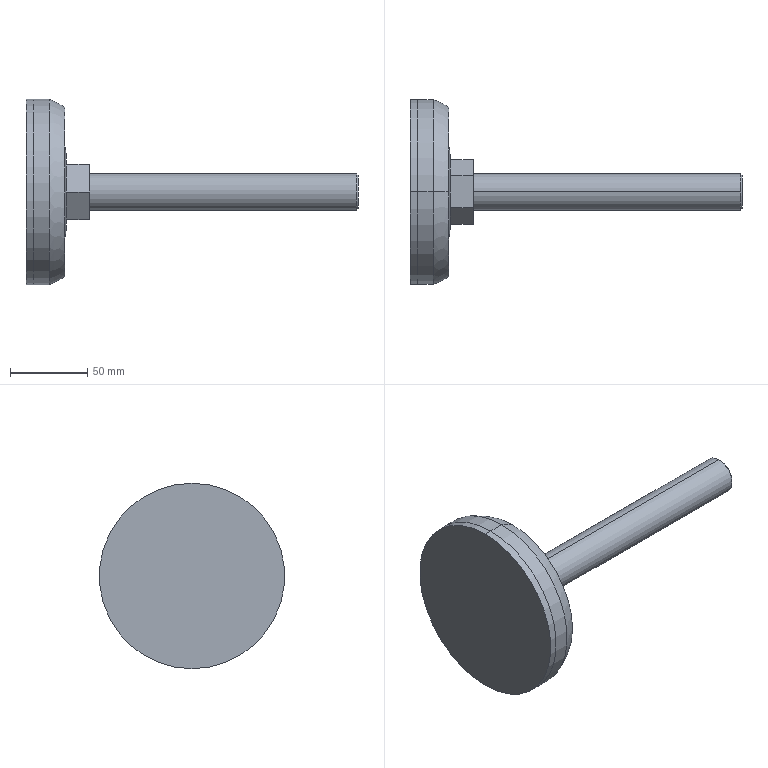Part | STEP file | 11-FJFN24_120pad11 | 2 solids | 27 faces | box 215 x 120 x 120 mm | volume 371412 mm3 | plane 13 | cylinder 8 | cone 4 | torus 2 | commonest cylinder face diameters 120 x4 24 x2 46.8 x2
STEP:
#1=CARTESIAN_POINT('',(-5.,0.,60.));
#2=VERTEX_POINT('',#1);
#3=CARTESIAN_POINT('',(-5.,0.,-60.));
#4=VERTEX_POINT('',#3);
#5=CARTESIAN_POINT('',(-5.,0.,0.));
#6=DIRECTION('',(-1.,0.,0.));
#7=DIRECTION('',(0.,0.,1.));
#8=AXIS2_PLACEMENT_3D('',#5,#6,#7);
#9=CIRCLE('',#8,60.);
#10=EDGE_CURVE('',#2,#4,#9,.T.);
#11=ORIENTED_EDGE('',*,*,#10,.F.);
#12=CARTESIAN_POINT('',(0.,0.,60.));
#13=VERTEX_POINT('',#12);
#14=CARTESIAN_POINT('',(-5.,0.,60.));
#15=DIRECTION('',(1.,0.,0.));
#16=VECTOR('',#15,1000.);
#17=LINE('',#14,#16);
#18=EDGE_CURVE('',#2,#13,#17,.T.);
#19=ORIENTED_EDGE('',*,*,#18,.T.);
#20=CARTESIAN_POINT('',(0.,0.,-60.));
#21=VERTEX_POINT('',#20);
#22=CARTESIAN_POINT('',(0.,0.,0.));
#23=DIRECTION('',(-1.,0.,0.));
#24=DIRECTION('',(0.,0.,1.));
#25=AXIS2_PLACEMENT_3D('',#22,#23,#24);
#26=CIRCLE('',#25,60.);
#27=EDGE_CURVE('',#13,#21,#26,.T.);
#28=ORIENTED_EDGE('',*,*,#27,.T.);
#29=CARTESIAN_POINT('',(-5.,0.,-60.));
#30=DIRECTION('',(1.,0.,0.));
#31=VECTOR('',#30,1000.);
#32=LINE('',#29,#31);
#33=EDGE_CURVE('',#4,#21,#32,.T.);
#34=ORIENTED_EDGE('',*,*,#33,.F.);
#35=EDGE_LOOP('',(#11,#19,#28,#34));
#36=FACE_OUTER_BOUND('',#35,.T.);
#37=CARTESIAN_POINT('',(-5.,0.,0.));
#38=DIRECTION('',(1.,0.,0.));
#39=DIRECTION('',(0.,0.,-1.));
#40=AXIS2_PLACEMENT_3D('',#37,#38,#39);
#41=CYLINDRICAL_SURFACE('',#40,60.);
#42=ADVANCED_FACE('',(#36),#41,.T.);
#43=ORIENTED_EDGE('',*,*,#18,.F.);
#44=CARTESIAN_POINT('',(-5.,0.,0.));
#45=DIRECTION('',(-1.,0.,0.));
#46=DIRECTION('',(0.,0.,1.));
#47=AXIS2_PLACEMENT_3D('',#44,#45,#46);
#48=CIRCLE('',#47,60.);
#49=EDGE_CURVE('',#4,#2,#48,.T.);
#50=ORIENTED_EDGE('',*,*,#49,.F.);
#51=ORIENTED_EDGE('',*,*,#33,.T.);
#52=CARTESIAN_POINT('',(0.,0.,0.));
#53=DIRECTION('',(-1.,0.,0.));
#54=DIRECTION('',(0.,0.,1.));
#55=AXIS2_PLACEMENT_3D('',#52,#53,#54);
#56=CIRCLE('',#55,60.);
#57=EDGE_CURVE('',#21,#13,#56,.T.);
#58=ORIENTED_EDGE('',*,*,#57,.T.);
#59=EDGE_LOOP('',(#43,#50,#51,#58));
#60=FACE_OUTER_BOUND('',#59,.T.);
#61=CARTESIAN_POINT('',(-5.,0.,0.));
#62=DIRECTION('',(1.,0.,0.));
#63=DIRECTION('',(0.,0.,-1.));
#64=AXIS2_PLACEMENT_3D('',#61,#62,#63);
#65=CYLINDRICAL_SURFACE('',#64,60.);
#66=ADVANCED_FACE('',(#60),#65,.T.);
#67=ORIENTED_EDGE('',*,*,#49,.T.);
#68=ORIENTED_EDGE('',*,*,#10,.T.);
#69=EDGE_LOOP('',(#67,#68));
#70=FACE_OUTER_BOUND('',#69,.T.);
#71=CARTESIAN_POINT('',(-5.,0.,0.));
#72=DIRECTION('',(-1.,0.,0.));
#73=DIRECTION('',(0.,0.,1.));
#74=AXIS2_PLACEMENT_3D('',#71,#72,#73);
#75=PLANE('',#74);
#76=ADVANCED_FACE('',(#70),#75,.T.);
#77=ORIENTED_EDGE('',*,*,#57,.F.);
#78=ORIENTED_EDGE('',*,*,#27,.F.);
#79=EDGE_LOOP('',(#77,#78));
#80=FACE_OUTER_BOUND('',#79,.T.);
#81=CARTESIAN_POINT('',(0.,0.,0.));
#82=DIRECTION('',(-1.,0.,0.));
#83=DIRECTION('',(0.,0.,1.));
#84=AXIS2_PLACEMENT_3D('',#81,#82,#83);
#85=PLANE('',#84);
#86=ADVANCED_FACE('',(#80),#85,.F.);
#87=CLOSED_SHELL('',(#42,#66,#76,#86));
#88=MANIFOLD_SOLID_BREP('',#87);
#89=CARTESIAN_POINT('',(210.,0.,-11.));
#90=VERTEX_POINT('',#89);
#91=CARTESIAN_POINT('',(210.,0.,11.));
#92=VERTEX_POINT('',#91);
#93=CARTESIAN_POINT('',(210.,0.,0.));
#94=DIRECTION('',(1.,0.,0.));
#95=DIRECTION('',(0.,0.,1.));
#96=AXIS2_PLACEMENT_3D('',#93,#94,#95);
#97=CIRCLE('',#96,11.);
#98=EDGE_CURVE('',#90,#92,#97,.T.);
#99=ORIENTED_EDGE('',*,*,#98,.F.);
#100=CARTESIAN_POINT('',(209.,0.,-12.));
#101=VERTEX_POINT('',#100);
#102=CARTESIAN_POINT('',(209.,0.,-12.));
#103=DIRECTION('',(-0.7071,0.,-0.7071));
#104=VECTOR('',#103,1000.);
#105=LINE('',#102,#104);
#106=EDGE_CURVE('',#90,#101,#105,.T.);
#107=ORIENTED_EDGE('',*,*,#106,.T.);
#108=CARTESIAN_POINT('',(209.,0.,12.));
#109=VERTEX_POINT('',#108);
#110=CARTESIAN_POINT('',(209.,0.,0.));
#111=DIRECTION('',(-1.,0.,0.));
#112=DIRECTION('',(0.,0.,1.));
#113=AXIS2_PLACEMENT_3D('',#110,#111,#112);
#114=CIRCLE('',#113,12.);
#115=EDGE_CURVE('',#109,#101,#114,.T.);
#116=ORIENTED_EDGE('',*,*,#115,.F.);
#117=CARTESIAN_POINT('',(209.,0.,12.));
#118=DIRECTION('',(-0.7071,0.,0.7071));
#119=VECTOR('',#118,1000.);
#120=LINE('',#117,#119);
#121=EDGE_CURVE('',#92,#109,#120,.T.);
#122=ORIENTED_EDGE('',*,*,#121,.F.);
#123=EDGE_LOOP('',(#99,#107,#116,#122));
#124=FACE_OUTER_BOUND('',#123,.T.);
#125=CARTESIAN_POINT('',(209.,0.,0.));
#126=DIRECTION('',(-1.,0.,0.));
#127=DIRECTION('',(0.,0.,1.));
#128=AXIS2_PLACEMENT_3D('',#125,#126,#127);
#129=CONICAL_SURFACE('',#128,12.,0.7854);
#130=ADVANCED_FACE('',(#124),#129,.T.);
#131=ORIENTED_EDGE('',*,*,#115,.T.);
#132=CARTESIAN_POINT('',(36.,0.,-12.));
#133=VERTEX_POINT('',#132);
#134=CARTESIAN_POINT('',(210.,0.,-12.));
#135=DIRECTION('',(-1.,0.,0.));
#136=VECTOR('',#135,1000.);
#137=LINE('',#134,#136);
#138=EDGE_CURVE('',#101,#133,#137,.T.);
#139=ORIENTED_EDGE('',*,*,#138,.T.);
#140=CARTESIAN_POINT('',(36.,0.,12.));
#141=VERTEX_POINT('',#140);
#142=CARTESIAN_POINT('',(36.,0.,0.));
#143=DIRECTION('',(-1.,0.,0.));
#144=DIRECTION('',(0.,0.,1.));
#145=AXIS2_PLACEMENT_3D('',#142,#143,#144);
#146=CIRCLE('',#145,12.);
#147=EDGE_CURVE('',#141,#133,#146,.T.);
#148=ORIENTED_EDGE('',*,*,#147,.F.);
#149=CARTESIAN_POINT('',(210.,0.,12.));
#150=DIRECTION('',(-1.,0.,0.));
#151=VECTOR('',#150,1000.);
#152=LINE('',#149,#151);
#153=EDGE_CURVE('',#109,#141,#152,.T.);
#154=ORIENTED_EDGE('',*,*,#153,.F.);
#155=EDGE_LOOP('',(#131,#139,#148,#154));
#156=FACE_OUTER_BOUND('',#155,.T.);
#157=CARTESIAN_POINT('',(210.,0.,0.));
#158=DIRECTION('',(-1.,0.,0.));
#159=DIRECTION('',(0.,0.,1.));
#160=AXIS2_PLACEMENT_3D('',#157,#158,#159);
#161=CYLINDRICAL_SURFACE('',#160,12.);
#162=ADVANCED_FACE('',(#156),#161,.T.);
#163=CARTESIAN_POINT('',(20.,0.,23.4));
#164=VERTEX_POINT('',#163);
#165=CARTESIAN_POINT('',(20.,0.,-23.4));
#166=VERTEX_POINT('',#165);
#167=CARTESIAN_POINT('',(20.,0.,0.));
#168=DIRECTION('',(1.,0.,0.));
#169=DIRECTION('',(0.,0.,-1.));
#170=AXIS2_PLACEMENT_3D('',#167,#168,#169);
#171=CIRCLE('',#170,23.4);
#172=EDGE_CURVE('',#164,#166,#171,.T.);
#173=ORIENTED_EDGE('',*,*,#172,.F.);
#174=CARTESIAN_POINT('',(21.206,0.,23.4));
#175=VERTEX_POINT('',#174);
#176=CARTESIAN_POINT('',(20.,0.,23.4));
#177=DIRECTION('',(1.,0.,0.));
#178=VECTOR('',#177,1000.);
#179=LINE('',#176,#178);
#180=EDGE_CURVE('',#164,#175,#179,.T.);
#181=ORIENTED_EDGE('',*,*,#180,.T.);
#182=CARTESIAN_POINT('',(21.206,0.,-23.4));
#183=VERTEX_POINT('',#182);
#184=CARTESIAN_POINT('',(21.206,0.,0.));
#185=DIRECTION('',(-1.,0.,0.));
#186=DIRECTION('',(0.,0.,1.));
#187=AXIS2_PLACEMENT_3D('',#184,#185,#186);
#188=CIRCLE('',#187,23.4);
#189=EDGE_CURVE('',#183,#175,#188,.T.);
#190=ORIENTED_EDGE('',*,*,#189,.F.);
#191=CARTESIAN_POINT('',(20.,0.,-23.4));
#192=DIRECTION('',(1.,0.,0.));
#193=VECTOR('',#192,1000.);
#194=LINE('',#191,#193);
#195=EDGE_CURVE('',#166,#183,#194,.T.);
#196=ORIENTED_EDGE('',*,*,#195,.F.);
#197=EDGE_LOOP('',(#173,#181,#190,#196));
#198=FACE_OUTER_BOUND('',#197,.T.);
#199=CARTESIAN_POINT('',(20.,0.,0.));
#200=DIRECTION('',(1.,0.,0.));
#201=DIRECTION('',(0.,0.,-1.));
#202=AXIS2_PLACEMENT_3D('',#199,#200,#201);
#203=CYLINDRICAL_SURFACE('',#202,23.4);
#204=ADVANCED_FACE('',(#198),#203,.F.);
#205=CARTESIAN_POINT('',(21.206,0.,0.));
#206=DIRECTION('',(-1.,0.,0.));
#207=DIRECTION('',(0.,0.,1.));
#208=AXIS2_PLACEMENT_3D('',#205,#206,#207);
#209=CIRCLE('',#208,23.4);
#210=EDGE_CURVE('',#175,#183,#209,.T.);
#211=ORIENTED_EDGE('',*,*,#210,.T.);
#212=CARTESIAN_POINT('',(20.,0.,-30.789));
#213=VERTEX_POINT('',#212);
#214=CARTESIAN_POINT('',(21.5,0.,-21.6));
#215=DIRECTION('',(-0.1611,0.,-0.9869));
#216=VECTOR('',#215,1000.);
#217=LINE('',#214,#216);
#218=EDGE_CURVE('',#183,#213,#217,.T.);
#219=ORIENTED_EDGE('',*,*,#218,.T.);
#220=CARTESIAN_POINT('',(20.,0.,30.789));
#221=VERTEX_POINT('',#220);
#222=CARTESIAN_POINT('',(20.,0.,0.));
#223=DIRECTION('',(-1.,0.,0.));
#224=DIRECTION('',(0.,0.,1.));
#225=AXIS2_PLACEMENT_3D('',#222,#223,#224);
#226=CIRCLE('',#225,30.789);
#227=EDGE_CURVE('',#221,#213,#226,.T.);
#228=ORIENTED_EDGE('',*,*,#227,.F.);
#229=CARTESIAN_POINT('',(21.5,0.,21.6));
#230=DIRECTION('',(-0.1611,0.,0.9869));
#231=VECTOR('',#230,1000.);
#232=LINE('',#229,#231);
#233=EDGE_CURVE('',#175,#221,#232,.T.);
#234=ORIENTED_EDGE('',*,*,#233,.F.);
#235=EDGE_LOOP('',(#211,#219,#228,#234));
#236=FACE_OUTER_BOUND('',#235,.T.);
#237=CARTESIAN_POINT('',(21.5,0.,0.));
#238=DIRECTION('',(-1.,0.,0.));
#239=DIRECTION('',(0.,0.,1.));
#240=AXIS2_PLACEMENT_3D('',#237,#238,#239);
#241=CONICAL_SURFACE('',#240,21.6,1.409);
#242=ADVANCED_FACE('',(#236),#241,.T.);
#243=CARTESIAN_POINT('',(20.,0.,54.885));
#244=VERTEX_POINT('',#243);
#245=CARTESIAN_POINT('',(20.,0.,-54.885));
#246=VERTEX_POINT('',#245);
#247=CARTESIAN_POINT('',(20.,0.,0.));
#248=DIRECTION('',(-1.,0.,0.));
#249=DIRECTION('',(0.,0.,1.));
#250=AXIS2_PLACEMENT_3D('',#247,#248,#249);
#251=CIRCLE('',#250,54.885);
#252=EDGE_CURVE('',#244,#246,#251,.T.);
#253=ORIENTED_EDGE('',*,*,#252,.T.);
#254=CARTESIAN_POINT('',(10.,0.,-60.));
#255=VERTEX_POINT('',#254);
#256=CARTESIAN_POINT('',(-13.736,0.,-1.264));
#257=DIRECTION('',(0.,1.,0.));
#258=DIRECTION('',(0.,0.,1.));
#259=AXIS2_PLACEMENT_3D('',#256,#257,#258);
#260=CIRCLE('',#259,63.351);
#261=EDGE_CURVE('',#246,#255,#260,.T.);
#262=ORIENTED_EDGE('',*,*,#261,.T.);
#263=CARTESIAN_POINT('',(10.,0.,60.));
#264=VERTEX_POINT('',#263);
#265=CARTESIAN_POINT('',(10.,0.,0.));
#266=DIRECTION('',(-1.,0.,0.));
#267=DIRECTION('',(0.,0.,1.));
#268=AXIS2_PLACEMENT_3D('',#265,#266,#267);
#269=CIRCLE('',#268,60.);
#270=EDGE_CURVE('',#264,#255,#269,.T.);
#271=ORIENTED_EDGE('',*,*,#270,.F.);
#272=CARTESIAN_POINT('',(-13.736,0.,1.264));
#273=DIRECTION('',(0.,-1.,0.));
#274=DIRECTION('',(0.,0.,-1.));
#275=AXIS2_PLACEMENT_3D('',#272,#273,#274);
#276=CIRCLE('',#275,63.351);
#277=EDGE_CURVE('',#244,#264,#276,.T.);
#278=ORIENTED_EDGE('',*,*,#277,.F.);
#279=EDGE_LOOP('',(#253,#262,#271,#278));
#280=FACE_OUTER_BOUND('',#279,.T.);
#281=CARTESIAN_POINT('',(-13.736,0.,0.));
#282=DIRECTION('',(-1.,0.,0.));
#283=DIRECTION('',(0.,0.,1.));
#284=AXIS2_PLACEMENT_3D('',#281,#282,#283);
#285=TOROIDAL_SURFACE('',#284,1.264,63.351);
#286=ADVANCED_FACE('',(#280),#285,.T.);
#287=ORIENTED_EDGE('',*,*,#270,.T.);
#288=CARTESIAN_POINT('',(0.,0.,-60.));
#289=VERTEX_POINT('',#288);
#290=CARTESIAN_POINT('',(210.,0.,-60.));
#291=DIRECTION('',(-1.,0.,0.));
#292=VECTOR('',#291,1000.);
#293=LINE('',#290,#292);
#294=EDGE_CURVE('',#255,#289,#293,.T.);
#295=ORIENTED_EDGE('',*,*,#294,.T.);
#296=CARTESIAN_POINT('',(0.,0.,60.));
#297=VERTEX_POINT('',#296);
#298=CARTESIAN_POINT('',(0.,0.,0.));
#299=DIRECTION('',(-1.,0.,0.));
#300=DIRECTION('',(0.,0.,1.));
#301=AXIS2_PLACEMENT_3D('',#298,#299,#300);
#302=CIRCLE('',#301,60.);
#303=EDGE_CURVE('',#297,#289,#302,.T.);
#304=ORIENTED_EDGE('',*,*,#303,.F.);
#305=CARTESIAN_POINT('',(210.,0.,60.));
#306=DIRECTION('',(-1.,0.,0.));
#307=VECTOR('',#306,1000.);
#308=LINE('',#305,#307);
#309=EDGE_CURVE('',#264,#297,#308,.T.);
#310=ORIENTED_EDGE('',*,*,#309,.F.);
#311=EDGE_LOOP('',(#287,#295,#304,#310));
#312=FACE_OUTER_BOUND('',#311,.T.);
#313=CARTESIAN_POINT('',(210.,0.,0.));
#314=DIRECTION('',(-1.,0.,0.));
#315=DIRECTION('',(0.,0.,1.));
#316=AXIS2_PLACEMENT_3D('',#313,#314,#315);
#317=CYLINDRICAL_SURFACE('',#316,60.);
#318=ADVANCED_FACE('',(#312),#317,.T.);
#319=ORIENTED_EDGE('',*,*,#303,.T.);
#320=CARTESIAN_POINT('',(0.,0.,0.));
#321=DIRECTION('',(-1.,0.,0.));
#322=DIRECTION('',(0.,0.,1.));
#323=AXIS2_PLACEMENT_3D('',#320,#321,#322);
#324=CIRCLE('',#323,60.);
#325=EDGE_CURVE('',#289,#297,#324,.T.);
#326=ORIENTED_EDGE('',*,*,#325,.T.);
#327=EDGE_LOOP('',(#319,#326));
#328=FACE_OUTER_BOUND('',#327,.T.);
#329=CARTESIAN_POINT('',(0.,0.,0.));
#330=DIRECTION('',(1.,0.,0.));
#331=DIRECTION('',(0.,0.,-1.));
#332=AXIS2_PLACEMENT_3D('',#329,#330,#331);
#333=PLANE('',#332);
#334=ADVANCED_FACE('',(#328),#333,.F.);
#335=ORIENTED_EDGE('',*,*,#294,.F.);
#336=CARTESIAN_POINT('',(10.,0.,0.));
#337=DIRECTION('',(-1.,0.,0.));
#338=DIRECTION('',(0.,0.,1.));
#339=AXIS2_PLACEMENT_3D('',#336,#337,#338);
#340=CIRCLE('',#339,60.);
#341=EDGE_CURVE('',#255,#264,#340,.T.);
#342=ORIENTED_EDGE('',*,*,#341,.T.);
#343=ORIENTED_EDGE('',*,*,#309,.T.);
#344=ORIENTED_EDGE('',*,*,#325,.F.);
#345=EDGE_LOOP('',(#335,#342,#343,#344));
#346=FACE_OUTER_BOUND('',#345,.T.);
#347=CARTESIAN_POINT('',(210.,0.,0.));
#348=DIRECTION('',(-1.,0.,0.));
#349=DIRECTION('',(0.,0.,1.));
#350=AXIS2_PLACEMENT_3D('',#347,#348,#349);
#351=CYLINDRICAL_SURFACE('',#350,60.);
#352=ADVANCED_FACE('',(#346),#351,.T.);
#353=ORIENTED_EDGE('',*,*,#261,.F.);
#354=CARTESIAN_POINT('',(20.,0.,0.));
#355=DIRECTION('',(-1.,0.,0.));
#356=DIRECTION('',(0.,0.,1.));
#357=AXIS2_PLACEMENT_3D('',#354,#355,#356);
#358=CIRCLE('',#357,54.885);
#359=EDGE_CURVE('',#246,#244,#358,.T.);
#360=ORIENTED_EDGE('',*,*,#359,.T.);
#361=ORIENTED_EDGE('',*,*,#277,.T.);
#362=ORIENTED_EDGE('',*,*,#341,.F.);
#363=EDGE_LOOP('',(#353,#360,#361,#362));
#364=FACE_OUTER_BOUND('',#363,.T.);
#365=CARTESIAN_POINT('',(-13.736,0.,0.));
#366=DIRECTION('',(-1.,0.,0.));
#367=DIRECTION('',(0.,0.,1.));
#368=AXIS2_PLACEMENT_3D('',#365,#366,#367);
#369=TOROIDAL_SURFACE('',#368,1.264,63.351);
#370=ADVANCED_FACE('',(#364),#369,.T.);
#371=ORIENTED_EDGE('',*,*,#252,.F.);
#372=ORIENTED_EDGE('',*,*,#359,.F.);
#373=EDGE_LOOP('',(#371,#372));
#374=FACE_OUTER_BOUND('',#373,.T.);
#375=ORIENTED_EDGE('',*,*,#227,.T.);
#376=CARTESIAN_POINT('',(20.,0.,0.));
#377=DIRECTION('',(-1.,0.,0.));
#378=DIRECTION('',(0.,0.,1.));
#379=AXIS2_PLACEMENT_3D('',#376,#377,#378);
#380=CIRCLE('',#379,30.789);
#381=EDGE_CURVE('',#213,#221,#380,.T.);
#382=ORIENTED_EDGE('',*,*,#381,.T.);
#383=EDGE_LOOP('',(#375,#382));
#384=FACE_BOUND('',#383,.T.);
#385=CARTESIAN_POINT('',(20.,54.885,0.));
#386=DIRECTION('',(-1.,0.,0.));
#387=DIRECTION('',(0.,0.,1.));
#388=AXIS2_PLACEMENT_3D('',#385,#386,#387);
#389=PLANE('',#388);
#390=ADVANCED_FACE('',(#374,#384),#389,.F.);
#391=ORIENTED_EDGE('',*,*,#218,.F.);
#392=ORIENTED_EDGE('',*,*,#189,.T.);
#393=ORIENTED_EDGE('',*,*,#233,.T.);
#394=ORIENTED_EDGE('',*,*,#381,.F.);
#395=EDGE_LOOP('',(#391,#392,#393,#394));
#396=FACE_OUTER_BOUND('',#395,.T.);
#397=CARTESIAN_POINT('',(21.5,0.,0.));
#398=DIRECTION('',(-1.,0.,0.));
#399=DIRECTION('',(0.,0.,1.));
#400=AXIS2_PLACEMENT_3D('',#397,#398,#399);
#401=CONICAL_SURFACE('',#400,21.6,1.409);
#402=ADVANCED_FACE('',(#396),#401,.T.);
#403=ORIENTED_EDGE('',*,*,#180,.F.);
#404=CARTESIAN_POINT('',(20.,0.,0.));
#405=DIRECTION('',(1.,0.,0.));
#406=DIRECTION('',(0.,0.,-1.));
#407=AXIS2_PLACEMENT_3D('',#404,#405,#406);
#408=CIRCLE('',#407,23.4);
#409=EDGE_CURVE('',#166,#164,#408,.T.);
#410=ORIENTED_EDGE('',*,*,#409,.F.);
#411=ORIENTED_EDGE('',*,*,#195,.T.);
#412=ORIENTED_EDGE('',*,*,#210,.F.);
#413=EDGE_LOOP('',(#403,#410,#411,#412));
#414=FACE_OUTER_BOUND('',#413,.T.);
#415=CARTESIAN_POINT('',(20.,0.,0.));
#416=DIRECTION('',(1.,0.,0.));
#417=DIRECTION('',(0.,0.,-1.));
#418=AXIS2_PLACEMENT_3D('',#415,#416,#417);
#419=CYLINDRICAL_SURFACE('',#418,23.4);
#420=ADVANCED_FACE('',(#414),#419,.F.);
#421=CARTESIAN_POINT('',(20.,10.392,-18.));
#422=VERTEX_POINT('',#421);
#423=CARTESIAN_POINT('',(20.,20.785,0.));
#424=VERTEX_POINT('',#423);
#425=CARTESIAN_POINT('',(20.,10.392,-18.));
#426=DIRECTION('',(0.,0.5,0.866));
#427=VECTOR('',#426,1000.);
#428=LINE('',#425,#427);
#429=EDGE_CURVE('',#422,#424,#428,.T.);
#430=ORIENTED_EDGE('',*,*,#429,.F.);
#431=CARTESIAN_POINT('',(20.,-10.392,-18.));
#432=VERTEX_POINT('',#431);
#433=CARTESIAN_POINT('',(20.,-10.392,-18.));
#434=DIRECTION('',(0.,1.,0.));
#435=VECTOR('',#434,1000.);
#436=LINE('',#433,#435);
#437=EDGE_CURVE('',#432,#422,#436,.T.);
#438=ORIENTED_EDGE('',*,*,#437,.F.);
#439=CARTESIAN_POINT('',(20.,-20.785,0.));
#440=VERTEX_POINT('',#439);
#441=CARTESIAN_POINT('',(20.,-20.785,0.));
#442=DIRECTION('',(0.,0.5,-0.866));
#443=VECTOR('',#442,1000.);
#444=LINE('',#441,#443);
#445=EDGE_CURVE('',#440,#432,#444,.T.);
#446=ORIENTED_EDGE('',*,*,#445,.F.);
#447=CARTESIAN_POINT('',(20.,-10.392,18.));
#448=VERTEX_POINT('',#447);
#449=CARTESIAN_POINT('',(20.,-10.392,18.));
#450=DIRECTION('',(0.,-0.5,-0.866));
#451=VECTOR('',#450,1000.);
#452=LINE('',#449,#451);
#453=EDGE_CURVE('',#448,#440,#452,.T.);
#454=ORIENTED_EDGE('',*,*,#453,.F.);
#455=CARTESIAN_POINT('',(20.,10.392,18.));
#456=VERTEX_POINT('',#455);
#457=CARTESIAN_POINT('',(20.,10.392,18.));
#458=DIRECTION('',(0.,-1.,0.));
#459=VECTOR('',#458,1000.);
#460=LINE('',#457,#459);
#461=EDGE_CURVE('',#456,#448,#460,.T.);
#462=ORIENTED_EDGE('',*,*,#461,.F.);
#463=CARTESIAN_POINT('',(20.,20.785,0.));
#464=DIRECTION('',(0.,-0.5,0.866));
#465=VECTOR('',#464,1000.);
#466=LINE('',#463,#465);
#467=EDGE_CURVE('',#424,#456,#466,.T.);
#468=ORIENTED_EDGE('',*,*,#467,.F.);
#469=EDGE_LOOP('',(#430,#438,#446,#454,#462,#468));
#470=FACE_BOUND('',#469,.T.);
#471=ORIENTED_EDGE('',*,*,#409,.T.);
#472=ORIENTED_EDGE('',*,*,#172,.T.);
#473=EDGE_LOOP('',(#471,#472));
#474=FACE_OUTER_BOUND('',#473,.T.);
#475=CARTESIAN_POINT('',(20.,0.,0.));
#476=DIRECTION('',(1.,0.,0.));
#477=DIRECTION('',(0.,0.,-1.));
#478=AXIS2_PLACEMENT_3D('',#475,#476,#477);
#479=PLANE('',#478);
#480=ADVANCED_FACE('',(#470,#474),#479,.T.);
#481=CARTESIAN_POINT('',(36.,20.785,0.));
#482=VERTEX_POINT('',#481);
#483=CARTESIAN_POINT('',(36.,10.392,18.));
#484=VERTEX_POINT('',#483);
#485=CARTESIAN_POINT('',(36.,20.785,0.));
#486=DIRECTION('',(0.,-0.5,0.866));
#487=VECTOR('',#486,1000.);
#488=LINE('',#485,#487);
#489=EDGE_CURVE('',#482,#484,#488,.T.);
#490=ORIENTED_EDGE('',*,*,#489,.F.);
#491=CARTESIAN_POINT('',(20.,20.785,0.));
#492=DIRECTION('',(1.,0.,0.));
#493=VECTOR('',#492,1000.);
#494=LINE('',#491,#493);
#495=EDGE_CURVE('',#424,#482,#494,.T.);
#496=ORIENTED_EDGE('',*,*,#495,.F.);
#497=ORIENTED_EDGE('',*,*,#467,.T.);
#498=CARTESIAN_POINT('',(20.,10.392,18.));
#499=DIRECTION('',(1.,0.,0.));
#500=VECTOR('',#499,1000.);
#501=LINE('',#498,#500);
#502=EDGE_CURVE('',#456,#484,#501,.T.);
#503=ORIENTED_EDGE('',*,*,#502,.T.);
#504=EDGE_LOOP('',(#490,#496,#497,#503));
#505=FACE_OUTER_BOUND('',#504,.T.);
#506=CARTESIAN_POINT('',(20.,20.785,0.));
#507=DIRECTION('',(0.,0.866,0.5));
#508=DIRECTION('',(0.,-0.5,0.866));
#509=AXIS2_PLACEMENT_3D('',#506,#507,#508);
#510=PLANE('',#509);
#511=ADVANCED_FACE('',(#505),#510,.T.);
#512=CARTESIAN_POINT('',(36.,10.392,-18.));
#513=VERTEX_POINT('',#512);
#514=CARTESIAN_POINT('',(36.,10.392,-18.));
#515=DIRECTION('',(0.,0.5,0.866));
#516=VECTOR('',#515,1000.);
#517=LINE('',#514,#516);
#518=EDGE_CURVE('',#513,#482,#517,.T.);
#519=ORIENTED_EDGE('',*,*,#518,.F.);
#520=CARTESIAN_POINT('',(20.,10.392,-18.));
#521=DIRECTION('',(1.,0.,0.));
#522=VECTOR('',#521,1000.);
#523=LINE('',#520,#522);
#524=EDGE_CURVE('',#422,#513,#523,.T.);
#525=ORIENTED_EDGE('',*,*,#524,.F.);
#526=ORIENTED_EDGE('',*,*,#429,.T.);
#527=ORIENTED_EDGE('',*,*,#495,.T.);
#528=EDGE_LOOP('',(#519,#525,#526,#527));
#529=FACE_OUTER_BOUND('',#528,.T.);
#530=CARTESIAN_POINT('',(20.,10.392,-18.));
#531=DIRECTION('',(0.,0.866,-0.5));
#532=DIRECTION('',(0.,0.5,0.866));
#533=AXIS2_PLACEMENT_3D('',#530,#531,#532);
#534=PLANE('',#533);
#535=ADVANCED_FACE('',(#529),#534,.T.);
#536=CARTESIAN_POINT('',(36.,-10.392,-18.));
#537=VERTEX_POINT('',#536);
#538=CARTESIAN_POINT('',(36.,-10.392,-18.));
#539=DIRECTION('',(0.,1.,0.));
#540=VECTOR('',#539,1000.);
#541=LINE('',#538,#540);
#542=EDGE_CURVE('',#537,#513,#541,.T.);
#543=ORIENTED_EDGE('',*,*,#542,.F.);
#544=CARTESIAN_POINT('',(20.,-10.392,-18.));
#545=DIRECTION('',(1.,0.,0.));
#546=VECTOR('',#545,1000.);
#547=LINE('',#544,#546);
#548=EDGE_CURVE('',#432,#537,#547,.T.);
#549=ORIENTED_EDGE('',*,*,#548,.F.);
#550=ORIENTED_EDGE('',*,*,#437,.T.);
#551=ORIENTED_EDGE('',*,*,#524,.T.);
#552=EDGE_LOOP('',(#543,#549,#550,#551));
#553=FACE_OUTER_BOUND('',#552,.T.);
#554=CARTESIAN_POINT('',(20.,-10.392,-18.));
#555=DIRECTION('',(0.,0.,-1.));
#556=DIRECTION('',(-1.,0.,0.));
#557=AXIS2_PLACEMENT_3D('',#554,#555,#556);
#558=PLANE('',#557);
#559=ADVANCED_FACE('',(#553),#558,.T.);
#560=CARTESIAN_POINT('',(36.,-20.785,0.));
#561=VERTEX_POINT('',#560);
#562=CARTESIAN_POINT('',(36.,-20.785,0.));
#563=DIRECTION('',(0.,0.5,-0.866));
#564=VECTOR('',#563,1000.);
#565=LINE('',#562,#564);
#566=EDGE_CURVE('',#561,#537,#565,.T.);
#567=ORIENTED_EDGE('',*,*,#566,.F.);
#568=CARTESIAN_POINT('',(20.,-20.785,0.));
#569=DIRECTION('',(1.,0.,0.));
#570=VECTOR('',#569,1000.);
#571=LINE('',#568,#570);
#572=EDGE_CURVE('',#440,#561,#571,.T.);
#573=ORIENTED_EDGE('',*,*,#572,.F.);
#574=ORIENTED_EDGE('',*,*,#445,.T.);
#575=ORIENTED_EDGE('',*,*,#548,.T.);
#576=EDGE_LOOP('',(#567,#573,#574,#575));
#577=FACE_OUTER_BOUND('',#576,.T.);
#578=CARTESIAN_POINT('',(20.,-20.785,0.));
#579=DIRECTION('',(0.,-0.866,-0.5));
#580=DIRECTION('',(0.,0.5,-0.866));
#581=AXIS2_PLACEMENT_3D('',#578,#579,#580);
#582=PLANE('',#581);
#583=ADVANCED_FACE('',(#577),#582,.T.);
#584=CARTESIAN_POINT('',(36.,-10.392,18.));
#585=VERTEX_POINT('',#584);
#586=CARTESIAN_POINT('',(36.,-10.392,18.));
#587=DIRECTION('',(0.,-0.5,-0.866));
#588=VECTOR('',#587,1000.);
#589=LINE('',#586,#588);
#590=EDGE_CURVE('',#585,#561,#589,.T.);
#591=ORIENTED_EDGE('',*,*,#590,.F.);
#592=CARTESIAN_POINT('',(20.,-10.392,18.));
#593=DIRECTION('',(1.,0.,0.));
#594=VECTOR('',#593,1000.);
#595=LINE('',#592,#594);
#596=EDGE_CURVE('',#448,#585,#595,.T.);
#597=ORIENTED_EDGE('',*,*,#596,.F.);
#598=ORIENTED_EDGE('',*,*,#453,.T.);
#599=ORIENTED_EDGE('',*,*,#572,.T.);
#600=EDGE_LOOP('',(#591,#597,#598,#599));
#601=FACE_OUTER_BOUND('',#600,.T.);
#602=CARTESIAN_POINT('',(20.,-10.392,18.));
#603=DIRECTION('',(0.,-0.866,0.5));
#604=DIRECTION('',(0.,-0.5,-0.866));
#605=AXIS2_PLACEMENT_3D('',#602,#603,#604);
#606=PLANE('',#605);
#607=ADVANCED_FACE('',(#601),#606,.T.);
#608=CARTESIAN_POINT('',(36.,10.392,18.));
#609=DIRECTION('',(0.,-1.,0.));
#610=VECTOR('',#609,1000.);
#611=LINE('',#608,#610);
#612=EDGE_CURVE('',#484,#585,#611,.T.);
#613=ORIENTED_EDGE('',*,*,#612,.F.);
#614=ORIENTED_EDGE('',*,*,#502,.F.);
#615=ORIENTED_EDGE('',*,*,#461,.T.);
#616=ORIENTED_EDGE('',*,*,#596,.T.);
#617=EDGE_LOOP('',(#613,#614,#615,#616));
#618=FACE_OUTER_BOUND('',#617,.T.);
#619=CARTESIAN_POINT('',(20.,10.392,18.));
#620=DIRECTION('',(0.,0.,1.));
#621=DIRECTION('',(1.,0.,0.));
#622=AXIS2_PLACEMENT_3D('',#619,#620,#621);
#623=PLANE('',#622);
#624=ADVANCED_FACE('',(#618),#623,.T.);
#625=CARTESIAN_POINT('',(210.,0.,0.));
#626=DIRECTION('',(1.,0.,0.));
#627=DIRECTION('',(0.,0.,1.));
#628=AXIS2_PLACEMENT_3D('',#625,#626,#627);
#629=CIRCLE('',#628,11.);
#630=EDGE_CURVE('',#92,#90,#629,.T.);
#631=ORIENTED_EDGE('',*,*,#630,.T.);
#632=ORIENTED_EDGE('',*,*,#98,.T.);
#633=EDGE_LOOP('',(#631,#632));
#634=FACE_OUTER_BOUND('',#633,.T.);
#635=CARTESIAN_POINT('',(210.,12.,0.));
#636=DIRECTION('',(-1.,0.,0.));
#637=DIRECTION('',(0.,0.,1.));
#638=AXIS2_PLACEMENT_3D('',#635,#636,#637);
#639=PLANE('',#638);
#640=ADVANCED_FACE('',(#634),#639,.F.);
#641=ORIENTED_EDGE('',*,*,#138,.F.);
#642=CARTESIAN_POINT('',(209.,0.,0.));
#643=DIRECTION('',(-1.,0.,0.));
#644=DIRECTION('',(0.,0.,1.));
#645=AXIS2_PLACEMENT_3D('',#642,#643,#644);
#646=CIRCLE('',#645,12.);
#647=EDGE_CURVE('',#101,#109,#646,.T.);
#648=ORIENTED_EDGE('',*,*,#647,.T.);
#649=ORIENTED_EDGE('',*,*,#153,.T.);
#650=CARTESIAN_POINT('',(36.,0.,0.));
#651=DIRECTION('',(-1.,0.,0.));
#652=DIRECTION('',(0.,0.,1.));
#653=AXIS2_PLACEMENT_3D('',#650,#651,#652);
#654=CIRCLE('',#653,12.);
#655=EDGE_CURVE('',#133,#141,#654,.T.);
#656=ORIENTED_EDGE('',*,*,#655,.F.);
#657=EDGE_LOOP('',(#641,#648,#649,#656));
#658=FACE_OUTER_BOUND('',#657,.T.);
#659=CARTESIAN_POINT('',(210.,0.,0.));
#660=DIRECTION('',(-1.,0.,0.));
#661=DIRECTION('',(0.,0.,1.));
#662=AXIS2_PLACEMENT_3D('',#659,#660,#661);
#663=CYLINDRICAL_SURFACE('',#662,12.);
#664=ADVANCED_FACE('',(#658),#663,.T.);
#665=ORIENTED_EDGE('',*,*,#147,.T.);
#666=ORIENTED_EDGE('',*,*,#655,.T.);
#667=EDGE_LOOP('',(#665,#666));
#668=FACE_BOUND('',#667,.T.);
#669=ORIENTED_EDGE('',*,*,#489,.T.);
#670=ORIENTED_EDGE('',*,*,#612,.T.);
#671=ORIENTED_EDGE('',*,*,#590,.T.);
#672=ORIENTED_EDGE('',*,*,#566,.T.);
#673=ORIENTED_EDGE('',*,*,#542,.T.);
#674=ORIENTED_EDGE('',*,*,#518,.T.);
#675=EDGE_LOOP('',(#669,#670,#671,#672,#673,#674));
#676=FACE_OUTER_BOUND('',#675,.T.);
#677=CARTESIAN_POINT('',(36.,21.6,0.));
#678=DIRECTION('',(-1.,0.,0.));
#679=DIRECTION('',(0.,0.,1.));
#680=AXIS2_PLACEMENT_3D('',#677,#678,#679);
#681=PLANE('',#680);
#682=ADVANCED_FACE('',(#668,#676),#681,.F.);
#683=ORIENTED_EDGE('',*,*,#106,.F.);
#684=ORIENTED_EDGE('',*,*,#630,.F.);
#685=ORIENTED_EDGE('',*,*,#121,.T.);
#686=ORIENTED_EDGE('',*,*,#647,.F.);
#687=EDGE_LOOP('',(#683,#684,#685,#686));
#688=FACE_OUTER_BOUND('',#687,.T.);
#689=CARTESIAN_POINT('',(209.,0.,0.));
#690=DIRECTION('',(-1.,0.,0.));
#691=DIRECTION('',(0.,0.,1.));
#692=AXIS2_PLACEMENT_3D('',#689,#690,#691);
#693=CONICAL_SURFACE('',#692,12.,0.7854);
#694=ADVANCED_FACE('',(#688),#693,.T.);
#695=CLOSED_SHELL('',(#130,#162,#204,#242,#286,#318,#334,#352,#370,#390,#402,#420,#480,#511,#535,#559,#583,#607,#624,#640,#664,#682,#694));
#696=MANIFOLD_SOLID_BREP('',#695);
#697=CARTESIAN_POINT('',(0.,0.,0.));
#698=DIRECTION('',(0.,0.,1.));
#699=DIRECTION('',(1.,0.,0.));
#700=AXIS2_PLACEMENT_3D('',#697,#698,#699);
#701=(LENGTH_UNIT()NAMED_UNIT(*)SI_UNIT(.MILLI.,.METRE.));
#702=UNCERTAINTY_MEASURE_WITH_UNIT(LENGTH_MEASURE(0.00001),#701,'','');
#703=(NAMED_UNIT(*)PLANE_ANGLE_UNIT()SI_UNIT($,.RADIAN.));
#704=(NAMED_UNIT(*)SI_UNIT($,.STERADIAN.)SOLID_ANGLE_UNIT());
#705=(GEOMETRIC_REPRESENTATION_CONTEXT(3)GLOBAL_UNCERTAINTY_ASSIGNED_CONTEXT((#702))GLOBAL_UNIT_ASSIGNED_CONTEXT((#701,#703,#704))REPRESENTATION_CONTEXT('',''));
#706=ADVANCED_BREP_SHAPE_REPRESENTATION('',(#88,#696,#700),#705);